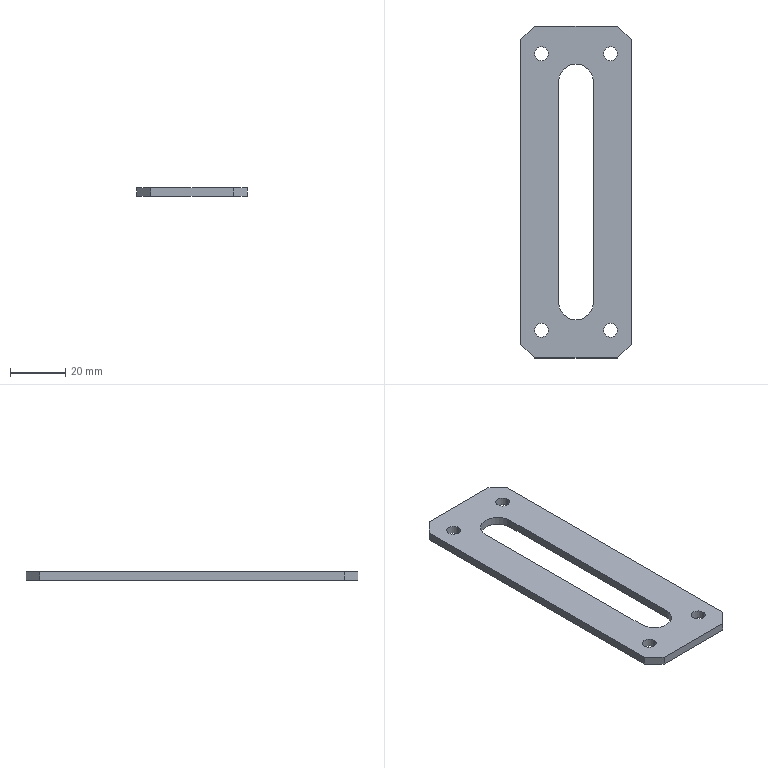Part | STEP file | Mounting Plate | 1 solid | 22 faces | box 40 x 120 x 3 mm | volume 10646 mm3 | plane 12 | cylinder 10 | commonest cylinder face diameters 5 x8 12.5 x2